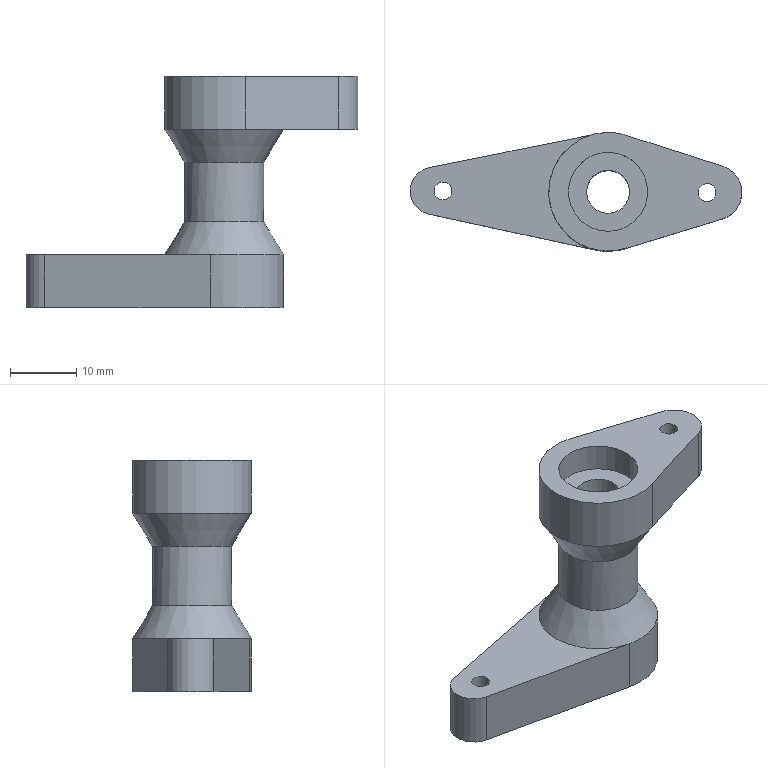Part | STEP file | Dodanie-wyci_gni_cie2 | 1 solid | 24 faces | box 50.275 x 17.999 x 35 mm | volume 7787 mm3 | cylinder 12 | plane 10 | cone 2 | commonest cylinder face diameters 17.999 x4 11.999 x3 2.7 x2 6.499 x1 7.152 x1 8.38 x1